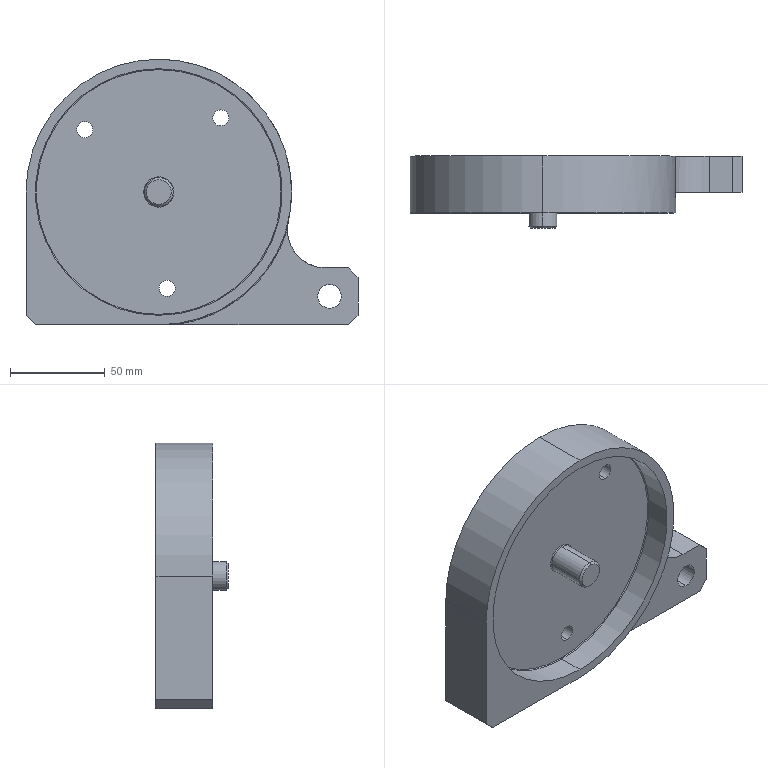Part | SolidWorks | features ICE 5, HoleWzd 2, Chamfer 1, Fillet 1, FlatPattern 1, SMBaseFlange 1, SheetMetal 1 | 1 solid | 49 faces | box 175 x 38 x 140 mm | volume 313299 mm3 | cylinder 21 | plane 13 | cone 8 | torus 7 | commonest cylinder face diameters 8.5 x10 12.5 x2 15 x2 83 x2 130 x2 140 x2
STEP:
#1=CARTESIAN_POINT('',(70.,-5.5,29.));
#2=VERTEX_POINT('',#1);
#3=CARTESIAN_POINT('',(70.,-5.5,111.));
#4=VERTEX_POINT('',#3);
#5=CARTESIAN_POINT('',(70.,-5.5,70.));
#6=DIRECTION('',(0.,1.,0.));
#7=DIRECTION('',(0.,0.,1.));
#8=AXIS2_PLACEMENT_3D('',#5,#6,#7);
#9=CIRCLE('',#8,41.);
#10=EDGE_CURVE('',#2,#4,#9,.T.);
#11=ORIENTED_EDGE('',*,*,#10,.F.);
#12=CARTESIAN_POINT('',(70.,-5.,28.5));
#13=VERTEX_POINT('',#12);
#14=CARTESIAN_POINT('',(70.,-5.,29.));
#15=DIRECTION('',(1.,0.,0.));
#16=DIRECTION('',(0.,0.,-1.));
#17=AXIS2_PLACEMENT_3D('',#14,#15,#16);
#18=CIRCLE('',#17,0.5);
#19=EDGE_CURVE('',#2,#13,#18,.T.);
#20=ORIENTED_EDGE('',*,*,#19,.T.);
#21=CARTESIAN_POINT('',(70.,-5.,111.5));
#22=VERTEX_POINT('',#21);
#23=CARTESIAN_POINT('',(70.,-5.,70.));
#24=DIRECTION('',(0.,-1.,0.));
#25=DIRECTION('',(0.,0.,1.));
#26=AXIS2_PLACEMENT_3D('',#23,#24,#25);
#27=CIRCLE('',#26,41.5);
#28=EDGE_CURVE('',#22,#13,#27,.T.);
#29=ORIENTED_EDGE('',*,*,#28,.F.);
#30=CARTESIAN_POINT('',(70.,-5.,111.));
#31=DIRECTION('',(-1.,0.,0.));
#32=DIRECTION('',(0.,0.,1.));
#33=AXIS2_PLACEMENT_3D('',#30,#31,#32);
#34=CIRCLE('',#33,0.5);
#35=EDGE_CURVE('',#4,#22,#34,.T.);
#36=ORIENTED_EDGE('',*,*,#35,.F.);
#37=EDGE_LOOP('',(#11,#20,#29,#36));
#38=FACE_OUTER_BOUND('',#37,.T.);
#39=CARTESIAN_POINT('',(70.,-5.,70.));
#40=DIRECTION('',(0.,1.,0.));
#41=DIRECTION('',(0.,0.,1.));
#42=AXIS2_PLACEMENT_3D('',#39,#40,#41);
#43=TOROIDAL_SURFACE('',#42,41.,0.5);
#44=ADVANCED_FACE('',(#38),#43,.F.);
#45=CARTESIAN_POINT('',(70.,-16.,134.5));
#46=VERTEX_POINT('',#45);
#47=CARTESIAN_POINT('',(70.,-16.,5.5));
#48=VERTEX_POINT('',#47);
#49=CARTESIAN_POINT('',(70.,-16.,70.));
#50=DIRECTION('',(0.,-1.,0.));
#51=DIRECTION('',(0.,0.,-1.));
#52=AXIS2_PLACEMENT_3D('',#49,#50,#51);
#53=CIRCLE('',#52,64.5);
#54=EDGE_CURVE('',#46,#48,#53,.T.);
#55=ORIENTED_EDGE('',*,*,#54,.F.);
#56=CARTESIAN_POINT('',(70.,-16.5,135.));
#57=VERTEX_POINT('',#56);
#58=CARTESIAN_POINT('',(70.,-16.5,134.5));
#59=DIRECTION('',(1.,0.,0.));
#60=DIRECTION('',(0.,0.,-1.));
#61=AXIS2_PLACEMENT_3D('',#58,#59,#60);
#62=CIRCLE('',#61,0.5);
#63=EDGE_CURVE('',#46,#57,#62,.T.);
#64=ORIENTED_EDGE('',*,*,#63,.T.);
#65=CARTESIAN_POINT('',(70.,-16.5,5.));
#66=VERTEX_POINT('',#65);
#67=CARTESIAN_POINT('',(70.,-16.5,70.));
#68=DIRECTION('',(0.,1.,0.));
#69=DIRECTION('',(0.,0.,-1.));
#70=AXIS2_PLACEMENT_3D('',#67,#68,#69);
#71=CIRCLE('',#70,65.);
#72=EDGE_CURVE('',#66,#57,#71,.T.);
#73=ORIENTED_EDGE('',*,*,#72,.F.);
#74=CARTESIAN_POINT('',(70.,-16.5,5.5));
#75=DIRECTION('',(-1.,0.,0.));
#76=DIRECTION('',(0.,0.,1.));
#77=AXIS2_PLACEMENT_3D('',#74,#75,#76);
#78=CIRCLE('',#77,0.5);
#79=EDGE_CURVE('',#48,#66,#78,.T.);
#80=ORIENTED_EDGE('',*,*,#79,.F.);
#81=EDGE_LOOP('',(#55,#64,#73,#80));
#82=FACE_OUTER_BOUND('',#81,.T.);
#83=CARTESIAN_POINT('',(70.,-16.5,70.));
#84=DIRECTION('',(0.,-1.,0.));
#85=DIRECTION('',(0.,0.,-1.));
#86=AXIS2_PLACEMENT_3D('',#83,#84,#85);
#87=TOROIDAL_SURFACE('',#86,64.5,0.5);
#88=ADVANCED_FACE('',(#82),#87,.F.);
#89=CARTESIAN_POINT('',(70.,-16.5,77.5));
#90=VERTEX_POINT('',#89);
#91=CARTESIAN_POINT('',(70.,-16.5,62.5));
#92=VERTEX_POINT('',#91);
#93=CARTESIAN_POINT('',(70.,-16.5,70.));
#94=DIRECTION('',(0.,-1.,0.));
#95=DIRECTION('',(0.,0.,-1.));
#96=AXIS2_PLACEMENT_3D('',#93,#94,#95);
#97=CIRCLE('',#96,7.5);
#98=EDGE_CURVE('',#90,#92,#97,.T.);
#99=ORIENTED_EDGE('',*,*,#98,.F.);
#100=CARTESIAN_POINT('',(70.,-16.,78.));
#101=VERTEX_POINT('',#100);
#102=CARTESIAN_POINT('',(70.,-16.5,78.));
#103=DIRECTION('',(1.,0.,0.));
#104=DIRECTION('',(0.,0.,-1.));
#105=AXIS2_PLACEMENT_3D('',#102,#103,#104);
#106=CIRCLE('',#105,0.5);
#107=EDGE_CURVE('',#90,#101,#106,.T.);
#108=ORIENTED_EDGE('',*,*,#107,.T.);
#109=CARTESIAN_POINT('',(70.,-16.,62.));
#110=VERTEX_POINT('',#109);
#111=CARTESIAN_POINT('',(70.,-16.,70.));
#112=DIRECTION('',(0.,1.,0.));
#113=DIRECTION('',(0.,0.,-1.));
#114=AXIS2_PLACEMENT_3D('',#111,#112,#113);
#115=CIRCLE('',#114,8.);
#116=EDGE_CURVE('',#110,#101,#115,.T.);
#117=ORIENTED_EDGE('',*,*,#116,.F.);
#118=CARTESIAN_POINT('',(70.,-16.5,62.));
#119=DIRECTION('',(-1.,0.,0.));
#120=DIRECTION('',(0.,0.,1.));
#121=AXIS2_PLACEMENT_3D('',#118,#119,#120);
#122=CIRCLE('',#121,0.5);
#123=EDGE_CURVE('',#92,#110,#122,.T.);
#124=ORIENTED_EDGE('',*,*,#123,.F.);
#125=EDGE_LOOP('',(#99,#108,#117,#124));
#126=FACE_OUTER_BOUND('',#125,.T.);
#127=CARTESIAN_POINT('',(70.,-16.5,70.));
#128=DIRECTION('',(0.,-1.,0.));
#129=DIRECTION('',(0.,0.,-1.));
#130=AXIS2_PLACEMENT_3D('',#127,#128,#129);
#131=TOROIDAL_SURFACE('',#130,8.,0.5);
#132=ADVANCED_FACE('',(#126),#131,.F.);
#133=CARTESIAN_POINT('',(70.,-1.,28.5));
#134=VERTEX_POINT('',#133);
#135=CARTESIAN_POINT('',(70.,-1.,111.5));
#136=VERTEX_POINT('',#135);
#137=CARTESIAN_POINT('',(70.,-1.,70.));
#138=DIRECTION('',(0.,1.,0.));
#139=DIRECTION('',(0.,0.,-1.));
#140=AXIS2_PLACEMENT_3D('',#137,#138,#139);
#141=CIRCLE('',#140,41.5);
#142=EDGE_CURVE('',#134,#136,#141,.T.);
#143=ORIENTED_EDGE('',*,*,#142,.F.);
#144=CARTESIAN_POINT('',(70.,0.,27.5));
#145=VERTEX_POINT('',#144);
#146=CARTESIAN_POINT('',(70.,-1.,28.5));
#147=DIRECTION('',(0.,0.7071,-0.7071));
#148=VECTOR('',#147,1000.);
#149=LINE('',#146,#148);
#150=EDGE_CURVE('',#134,#145,#149,.T.);
#151=ORIENTED_EDGE('',*,*,#150,.T.);
#152=CARTESIAN_POINT('',(70.,0.,112.5));
#153=VERTEX_POINT('',#152);
#154=CARTESIAN_POINT('',(70.,0.,70.));
#155=DIRECTION('',(0.,-1.,0.));
#156=DIRECTION('',(0.,0.,-1.));
#157=AXIS2_PLACEMENT_3D('',#154,#155,#156);
#158=CIRCLE('',#157,42.5);
#159=EDGE_CURVE('',#153,#145,#158,.T.);
#160=ORIENTED_EDGE('',*,*,#159,.F.);
#161=CARTESIAN_POINT('',(70.,-1.,111.5));
#162=DIRECTION('',(0.,0.7071,0.7071));
#163=VECTOR('',#162,1000.);
#164=LINE('',#161,#163);
#165=EDGE_CURVE('',#136,#153,#164,.T.);
#166=ORIENTED_EDGE('',*,*,#165,.F.);
#167=EDGE_LOOP('',(#143,#151,#160,#166));
#168=FACE_OUTER_BOUND('',#167,.T.);
#169=CARTESIAN_POINT('',(70.,-1.,70.));
#170=DIRECTION('',(0.,1.,0.));
#171=DIRECTION('',(0.,0.,1.));
#172=AXIS2_PLACEMENT_3D('',#169,#170,#171);
#173=CONICAL_SURFACE('',#172,41.5,0.7854);
#174=ADVANCED_FACE('',(#168),#173,.F.);
#175=CARTESIAN_POINT('',(70.,-38.,63.5));
#176=VERTEX_POINT('',#175);
#177=CARTESIAN_POINT('',(70.,-38.,76.5));
#178=VERTEX_POINT('',#177);
#179=CARTESIAN_POINT('',(70.,-38.,70.));
#180=DIRECTION('',(0.,-1.,0.));
#181=DIRECTION('',(0.,0.,-1.));
#182=AXIS2_PLACEMENT_3D('',#179,#180,#181);
#183=CIRCLE('',#182,6.5);
#184=EDGE_CURVE('',#176,#178,#183,.T.);
#185=ORIENTED_EDGE('',*,*,#184,.F.);
#186=CARTESIAN_POINT('',(70.,-37.,62.5));
#187=VERTEX_POINT('',#186);
#188=CARTESIAN_POINT('',(70.,-38.,63.5));
#189=DIRECTION('',(0.,0.7071,-0.7071));
#190=VECTOR('',#189,1000.);
#191=LINE('',#188,#190);
#192=EDGE_CURVE('',#176,#187,#191,.T.);
#193=ORIENTED_EDGE('',*,*,#192,.T.);
#194=CARTESIAN_POINT('',(70.,-37.,77.5));
#195=VERTEX_POINT('',#194);
#196=CARTESIAN_POINT('',(70.,-37.,70.));
#197=DIRECTION('',(0.,1.,0.));
#198=DIRECTION('',(0.,0.,-1.));
#199=AXIS2_PLACEMENT_3D('',#196,#197,#198);
#200=CIRCLE('',#199,7.5);
#201=EDGE_CURVE('',#195,#187,#200,.T.);
#202=ORIENTED_EDGE('',*,*,#201,.F.);
#203=CARTESIAN_POINT('',(70.,-38.,76.5));
#204=DIRECTION('',(0.,0.7071,0.7071));
#205=VECTOR('',#204,1000.);
#206=LINE('',#203,#205);
#207=EDGE_CURVE('',#178,#195,#206,.T.);
#208=ORIENTED_EDGE('',*,*,#207,.F.);
#209=EDGE_LOOP('',(#185,#193,#202,#208));
#210=FACE_OUTER_BOUND('',#209,.T.);
#211=CARTESIAN_POINT('',(70.,-38.,70.));
#212=DIRECTION('',(0.,1.,0.));
#213=DIRECTION('',(0.,0.,1.));
#214=AXIS2_PLACEMENT_3D('',#211,#212,#213);
#215=CONICAL_SURFACE('',#214,6.5,0.7854);
#216=ADVANCED_FACE('',(#210),#215,.T.);
#217=CARTESIAN_POINT('',(19.25,-9.5,23.));
#218=VERTEX_POINT('',#217);
#219=CARTESIAN_POINT('',(10.75,-9.5,23.));
#220=VERTEX_POINT('',#219);
#221=CARTESIAN_POINT('',(15.,-9.5,23.));
#222=DIRECTION('',(0.,0.,-1.));
#223=DIRECTION('',(-1.,0.,0.));
#224=AXIS2_PLACEMENT_3D('',#221,#222,#223);
#225=CIRCLE('',#224,4.25);
#226=EDGE_CURVE('',#218,#220,#225,.T.);
#227=ORIENTED_EDGE('',*,*,#226,.F.);
#228=CARTESIAN_POINT('',(19.25,-9.5,0.));
#229=VERTEX_POINT('',#228);
#230=CARTESIAN_POINT('',(19.25,-9.5,0.));
#231=DIRECTION('',(0.,0.,-1.));
#232=VECTOR('',#231,1000.);
#233=LINE('',#230,#232);
#234=EDGE_CURVE('',#218,#229,#233,.T.);
#235=ORIENTED_EDGE('',*,*,#234,.T.);
#236=CARTESIAN_POINT('',(10.75,-9.5,0.));
#237=VERTEX_POINT('',#236);
#238=CARTESIAN_POINT('',(15.,-9.5,0.));
#239=DIRECTION('',(0.,0.,-1.));
#240=DIRECTION('',(-1.,0.,0.));
#241=AXIS2_PLACEMENT_3D('',#238,#239,#240);
#242=CIRCLE('',#241,4.25);
#243=EDGE_CURVE('',#229,#237,#242,.T.);
#244=ORIENTED_EDGE('',*,*,#243,.T.);
#245=CARTESIAN_POINT('',(10.75,-9.5,0.));
#246=DIRECTION('',(0.,0.,-1.));
#247=VECTOR('',#246,1000.);
#248=LINE('',#245,#247);
#249=EDGE_CURVE('',#220,#237,#248,.T.);
#250=ORIENTED_EDGE('',*,*,#249,.F.);
#251=EDGE_LOOP('',(#227,#235,#244,#250));
#252=FACE_OUTER_BOUND('',#251,.T.);
#253=CARTESIAN_POINT('',(15.,-9.5,0.));
#254=DIRECTION('',(0.,0.,-1.));
#255=DIRECTION('',(-1.,0.,0.));
#256=AXIS2_PLACEMENT_3D('',#253,#254,#255);
#257=CYLINDRICAL_SURFACE('',#256,4.25);
#258=ADVANCED_FACE('',(#252),#257,.F.);
#259=CARTESIAN_POINT('',(15.,-9.5,25.554));
#260=VERTEX_POINT('',#259);
#261=CARTESIAN_POINT('',(10.75,-9.5,23.));
#262=DIRECTION('',(-0.8572,0.,-0.515));
#263=VECTOR('',#262,1000.);
#264=LINE('',#261,#263);
#265=EDGE_CURVE('',#260,#220,#264,.T.);
#266=ORIENTED_EDGE('',*,*,#265,.F.);
#267=CARTESIAN_POINT('',(19.25,-9.5,23.));
#268=DIRECTION('',(0.8572,0.,-0.515));
#269=VECTOR('',#268,1000.);
#270=LINE('',#267,#269);
#271=EDGE_CURVE('',#260,#218,#270,.T.);
#272=ORIENTED_EDGE('',*,*,#271,.T.);
#273=ORIENTED_EDGE('',*,*,#226,.T.);
#274=EDGE_LOOP('',(#266,#272,#273));
#275=FACE_OUTER_BOUND('',#274,.T.);
#276=CARTESIAN_POINT('',(15.,-9.5,23.));
#277=DIRECTION('',(0.,0.,-1.));
#278=DIRECTION('',(-1.,0.,0.));
#279=AXIS2_PLACEMENT_3D('',#276,#277,#278);
#280=CONICAL_SURFACE('',#279,4.25,1.03);
#281=ADVANCED_FACE('',(#275),#280,.F.);
#282=CARTESIAN_POINT('',(134.25,-9.5,23.));
#283=VERTEX_POINT('',#282);
#284=CARTESIAN_POINT('',(125.75,-9.5,23.));
#285=VERTEX_POINT('',#284);
#286=CARTESIAN_POINT('',(130.,-9.5,23.));
#287=DIRECTION('',(0.,0.,-1.));
#288=DIRECTION('',(-1.,0.,0.));
#289=AXIS2_PLACEMENT_3D('',#286,#287,#288);
#290=CIRCLE('',#289,4.25);
#291=EDGE_CURVE('',#283,#285,#290,.T.);
#292=ORIENTED_EDGE('',*,*,#291,.F.);
#293=CARTESIAN_POINT('',(134.25,-9.5,0.));
#294=VERTEX_POINT('',#293);
#295=CARTESIAN_POINT('',(134.25,-9.5,0.));
#296=DIRECTION('',(0.,0.,-1.));
#297=VECTOR('',#296,1000.);
#298=LINE('',#295,#297);
#299=EDGE_CURVE('',#283,#294,#298,.T.);
#300=ORIENTED_EDGE('',*,*,#299,.T.);
#301=CARTESIAN_POINT('',(125.75,-9.5,0.));
#302=VERTEX_POINT('',#301);
#303=CARTESIAN_POINT('',(130.,-9.5,0.));
#304=DIRECTION('',(0.,0.,-1.));
#305=DIRECTION('',(-1.,0.,0.));
#306=AXIS2_PLACEMENT_3D('',#303,#304,#305);
#307=CIRCLE('',#306,4.25);
#308=EDGE_CURVE('',#294,#302,#307,.T.);
#309=ORIENTED_EDGE('',*,*,#308,.T.);
#310=CARTESIAN_POINT('',(125.75,-9.5,0.));
#311=DIRECTION('',(0.,0.,-1.));
#312=VECTOR('',#311,1000.);
#313=LINE('',#310,#312);
#314=EDGE_CURVE('',#285,#302,#313,.T.);
#315=ORIENTED_EDGE('',*,*,#314,.F.);
#316=EDGE_LOOP('',(#292,#300,#309,#315));
#317=FACE_OUTER_BOUND('',#316,.T.);
#318=CARTESIAN_POINT('',(130.,-9.5,0.));
#319=DIRECTION('',(0.,0.,-1.));
#320=DIRECTION('',(-1.,0.,0.));
#321=AXIS2_PLACEMENT_3D('',#318,#319,#320);
#322=CYLINDRICAL_SURFACE('',#321,4.25);
#323=ADVANCED_FACE('',(#317),#322,.F.);
#324=CARTESIAN_POINT('',(130.,-9.5,25.554));
#325=VERTEX_POINT('',#324);
#326=CARTESIAN_POINT('',(125.75,-9.5,23.));
#327=DIRECTION('',(-0.8572,0.,-0.515));
#328=VECTOR('',#327,1000.);
#329=LINE('',#326,#328);
#330=EDGE_CURVE('',#325,#285,#329,.T.);
#331=ORIENTED_EDGE('',*,*,#330,.F.);
#332=CARTESIAN_POINT('',(134.25,-9.5,23.));
#333=DIRECTION('',(0.8572,0.,-0.515));
#334=VECTOR('',#333,1000.);
#335=LINE('',#332,#334);
#336=EDGE_CURVE('',#325,#283,#335,.T.);
#337=ORIENTED_EDGE('',*,*,#336,.T.);
#338=ORIENTED_EDGE('',*,*,#291,.T.);
#339=EDGE_LOOP('',(#331,#337,#338));
#340=FACE_OUTER_BOUND('',#339,.T.);
#341=CARTESIAN_POINT('',(130.,-9.5,23.));
#342=DIRECTION('',(0.,0.,-1.));
#343=DIRECTION('',(-1.,0.,0.));
#344=AXIS2_PLACEMENT_3D('',#341,#342,#343);
#345=CONICAL_SURFACE('',#344,4.25,1.03);
#346=ADVANCED_FACE('',(#340),#345,.F.);
#347=CARTESIAN_POINT('',(102.782,-16.,113.318));
#348=VERTEX_POINT('',#347);
#349=CARTESIAN_POINT('',(102.782,-16.,104.818));
#350=VERTEX_POINT('',#349);
#351=CARTESIAN_POINT('',(102.782,-16.,109.068));
#352=DIRECTION('',(0.,-1.,0.));
#353=DIRECTION('',(0.,0.,-1.));
#354=AXIS2_PLACEMENT_3D('',#351,#352,#353);
#355=CIRCLE('',#354,4.25);
#356=EDGE_CURVE('',#348,#350,#355,.T.);
#357=ORIENTED_EDGE('',*,*,#356,.T.);
#358=CARTESIAN_POINT('',(102.782,0.,104.818));
#359=VERTEX_POINT('',#358);
#360=CARTESIAN_POINT('',(102.782,0.,104.818));
#361=DIRECTION('',(0.,1.,0.));
#362=VECTOR('',#361,1000.);
#363=LINE('',#360,#362);
#364=EDGE_CURVE('',#350,#359,#363,.T.);
#365=ORIENTED_EDGE('',*,*,#364,.T.);
#366=CARTESIAN_POINT('',(102.782,0.,113.318));
#367=VERTEX_POINT('',#366);
#368=CARTESIAN_POINT('',(102.782,0.,109.068));
#369=DIRECTION('',(0.,1.,0.));
#370=DIRECTION('',(0.,0.,1.));
#371=AXIS2_PLACEMENT_3D('',#368,#369,#370);
#372=CIRCLE('',#371,4.25);
#373=EDGE_CURVE('',#359,#367,#372,.T.);
#374=ORIENTED_EDGE('',*,*,#373,.T.);
#375=CARTESIAN_POINT('',(102.782,0.,113.318));
#376=DIRECTION('',(0.,1.,0.));
#377=VECTOR('',#376,1000.);
#378=LINE('',#375,#377);
#379=EDGE_CURVE('',#348,#367,#378,.T.);
#380=ORIENTED_EDGE('',*,*,#379,.F.);
#381=EDGE_LOOP('',(#357,#365,#374,#380));
#382=FACE_OUTER_BOUND('',#381,.T.);
#383=CARTESIAN_POINT('',(102.782,0.,109.068));
#384=DIRECTION('',(0.,1.,0.));
#385=DIRECTION('',(0.,0.,1.));
#386=AXIS2_PLACEMENT_3D('',#383,#384,#385);
#387=CYLINDRICAL_SURFACE('',#386,4.25);
#388=ADVANCED_FACE('',(#382),#387,.F.);
#389=CARTESIAN_POINT('',(74.445,-16.,23.444));
#390=VERTEX_POINT('',#389);
#391=CARTESIAN_POINT('',(74.445,-16.,14.944));
#392=VERTEX_POINT('',#391);
#393=CARTESIAN_POINT('',(74.445,-16.,19.194));
#394=DIRECTION('',(0.,-1.,0.));
#395=DIRECTION('',(0.,0.,-1.));
#396=AXIS2_PLACEMENT_3D('',#393,#394,#395);
#397=CIRCLE('',#396,4.25);
#398=EDGE_CURVE('',#390,#392,#397,.T.);
#399=ORIENTED_EDGE('',*,*,#398,.T.);
#400=CARTESIAN_POINT('',(74.445,0.,14.944));
#401=VERTEX_POINT('',#400);
#402=CARTESIAN_POINT('',(74.445,0.,14.944));
#403=DIRECTION('',(0.,1.,0.));
#404=VECTOR('',#403,1000.);
#405=LINE('',#402,#404);
#406=EDGE_CURVE('',#392,#401,#405,.T.);
#407=ORIENTED_EDGE('',*,*,#406,.T.);
#408=CARTESIAN_POINT('',(74.445,0.,23.444));
#409=VERTEX_POINT('',#408);
#410=CARTESIAN_POINT('',(74.445,0.,19.194));
#411=DIRECTION('',(0.,1.,0.));
#412=DIRECTION('',(0.,0.,1.));
#413=AXIS2_PLACEMENT_3D('',#410,#411,#412);
#414=CIRCLE('',#413,4.25);
#415=EDGE_CURVE('',#401,#409,#414,.T.);
#416=ORIENTED_EDGE('',*,*,#415,.T.);
#417=CARTESIAN_POINT('',(74.445,0.,23.444));
#418=DIRECTION('',(0.,1.,0.));
#419=VECTOR('',#418,1000.);
#420=LINE('',#417,#419);
#421=EDGE_CURVE('',#390,#409,#420,.T.);
#422=ORIENTED_EDGE('',*,*,#421,.F.);
#423=EDGE_LOOP('',(#399,#407,#416,#422));
#424=FACE_OUTER_BOUND('',#423,.T.);
#425=CARTESIAN_POINT('',(74.445,0.,19.194));
#426=DIRECTION('',(0.,1.,0.));
#427=DIRECTION('',(0.,0.,1.));
#428=AXIS2_PLACEMENT_3D('',#425,#426,#427);
#429=CYLINDRICAL_SURFACE('',#428,4.25);
#430=ADVANCED_FACE('',(#424),#429,.F.);
#431=CARTESIAN_POINT('',(30.932,-16.,107.032));
#432=VERTEX_POINT('',#431);
#433=CARTESIAN_POINT('',(30.932,-16.,98.532));
#434=VERTEX_POINT('',#433);
#435=CARTESIAN_POINT('',(30.932,-16.,102.782));
#436=DIRECTION('',(0.,-1.,0.));
#437=DIRECTION('',(0.,0.,-1.));
#438=AXIS2_PLACEMENT_3D('',#435,#436,#437);
#439=CIRCLE('',#438,4.25);
#440=EDGE_CURVE('',#432,#434,#439,.T.);
#441=ORIENTED_EDGE('',*,*,#440,.T.);
#442=CARTESIAN_POINT('',(30.932,0.,98.532));
#443=VERTEX_POINT('',#442);
#444=CARTESIAN_POINT('',(30.932,0.,98.532));
#445=DIRECTION('',(0.,1.,0.));
#446=VECTOR('',#445,1000.);
#447=LINE('',#444,#446);
#448=EDGE_CURVE('',#434,#443,#447,.T.);
#449=ORIENTED_EDGE('',*,*,#448,.T.);
#450=CARTESIAN_POINT('',(30.932,0.,107.032));
#451=VERTEX_POINT('',#450);
#452=CARTESIAN_POINT('',(30.932,0.,102.782));
#453=DIRECTION('',(0.,1.,0.));
#454=DIRECTION('',(0.,0.,1.));
#455=AXIS2_PLACEMENT_3D('',#452,#453,#454);
#456=CIRCLE('',#455,4.25);
#457=EDGE_CURVE('',#443,#451,#456,.T.);
#458=ORIENTED_EDGE('',*,*,#457,.T.);
#459=CARTESIAN_POINT('',(30.932,0.,107.032));
#460=DIRECTION('',(0.,1.,0.));
#461=VECTOR('',#460,1000.);
#462=LINE('',#459,#461);
#463=EDGE_CURVE('',#432,#451,#462,.T.);
#464=ORIENTED_EDGE('',*,*,#463,.F.);
#465=EDGE_LOOP('',(#441,#449,#458,#464));
#466=FACE_OUTER_BOUND('',#465,.T.);
#467=CARTESIAN_POINT('',(30.932,0.,102.782));
#468=DIRECTION('',(0.,1.,0.));
#469=DIRECTION('',(0.,0.,1.));
#470=AXIS2_PLACEMENT_3D('',#467,#468,#469);
#471=CYLINDRICAL_SURFACE('',#470,4.25);
#472=ADVANCED_FACE('',(#466),#471,.F.);
#473=ORIENTED_EDGE('',*,*,#28,.T.);
#474=CARTESIAN_POINT('',(70.,-5.5,28.5));
#475=DIRECTION('',(0.,1.,0.));
#476=VECTOR('',#475,1000.);
#477=LINE('',#474,#476);
#478=EDGE_CURVE('',#13,#134,#477,.T.);
#479=ORIENTED_EDGE('',*,*,#478,.T.);
#480=ORIENTED_EDGE('',*,*,#142,.T.);
#481=CARTESIAN_POINT('',(70.,-5.5,111.5));
#482=DIRECTION('',(0.,1.,0.));
#483=VECTOR('',#482,1000.);
#484=LINE('',#481,#483);
#485=EDGE_CURVE('',#22,#136,#484,.T.);
#486=ORIENTED_EDGE('',*,*,#485,.F.);
#487=EDGE_LOOP('',(#473,#479,#480,#486));
#488=FACE_OUTER_BOUND('',#487,.T.);
#489=CARTESIAN_POINT('',(70.,-5.5,70.));
#490=DIRECTION('',(0.,1.,0.));
#491=DIRECTION('',(0.,0.,1.));
#492=AXIS2_PLACEMENT_3D('',#489,#490,#491);
#493=CYLINDRICAL_SURFACE('',#492,41.5);
#494=ADVANCED_FACE('',(#488),#493,.F.);
#495=CARTESIAN_POINT('',(70.,-16.5,70.));
#496=DIRECTION('',(0.,-1.,0.));
#497=DIRECTION('',(0.,0.,-1.));
#498=AXIS2_PLACEMENT_3D('',#495,#496,#497);
#499=CIRCLE('',#498,7.5);
#500=EDGE_CURVE('',#92,#90,#499,.T.);
#501=ORIENTED_EDGE('',*,*,#500,.T.);
#502=CARTESIAN_POINT('',(70.,-16.,77.5));
#503=DIRECTION('',(0.,-1.,0.));
#504=VECTOR('',#503,1000.);
#505=LINE('',#502,#504);
#506=EDGE_CURVE('',#90,#195,#505,.T.);
#507=ORIENTED_EDGE('',*,*,#506,.T.);
#508=ORIENTED_EDGE('',*,*,#201,.T.);
#509=CARTESIAN_POINT('',(70.,-16.,62.5));
#510=DIRECTION('',(0.,-1.,0.));
#511=VECTOR('',#510,1000.);
#512=LINE('',#509,#511);
#513=EDGE_CURVE('',#92,#187,#512,.T.);
#514=ORIENTED_EDGE('',*,*,#513,.F.);
#515=EDGE_LOOP('',(#501,#507,#508,#514));
#516=FACE_OUTER_BOUND('',#515,.T.);
#517=CARTESIAN_POINT('',(70.,-16.,70.));
#518=DIRECTION('',(0.,-1.,0.));
#519=DIRECTION('',(0.,0.,-1.));
#520=AXIS2_PLACEMENT_3D('',#517,#518,#519);
#521=CYLINDRICAL_SURFACE('',#520,7.5);
#522=ADVANCED_FACE('',(#516),#521,.T.);
#523=ORIENTED_EDGE('',*,*,#72,.T.);
#524=CARTESIAN_POINT('',(70.,-30.,135.));
#525=VERTEX_POINT('',#524);
#526=CARTESIAN_POINT('',(70.,-16.,135.));
#527=DIRECTION('',(0.,-1.,0.));
#528=VECTOR('',#527,1000.);
#529=LINE('',#526,#528);
#530=EDGE_CURVE('',#57,#525,#529,.T.);
#531=ORIENTED_EDGE('',*,*,#530,.T.);
#532=CARTESIAN_POINT('',(70.,-30.,5.));
#533=VERTEX_POINT('',#532);
#534=CARTESIAN_POINT('',(70.,-30.,70.));
#535=DIRECTION('',(0.,-1.,0.));
#536=DIRECTION('',(0.,0.,-1.));
#537=AXIS2_PLACEMENT_3D('',#534,#535,#536);
#538=CIRCLE('',#537,65.);
#539=EDGE_CURVE('',#525,#533,#538,.T.);
#540=ORIENTED_EDGE('',*,*,#539,.T.);
#541=CARTESIAN_POINT('',(70.,-16.,5.));
#542=DIRECTION('',(0.,-1.,0.));
#543=VECTOR('',#542,1000.);
#544=LINE('',#541,#543);
#545=EDGE_CURVE('',#66,#533,#544,.T.);
#546=ORIENTED_EDGE('',*,*,#545,.F.);
#547=EDGE_LOOP('',(#523,#531,#540,#546));
#548=FACE_OUTER_BOUND('',#547,.T.);
#549=CARTESIAN_POINT('',(70.,-16.,70.));
#550=DIRECTION('',(0.,-1.,0.));
#551=DIRECTION('',(0.,0.,-1.));
#552=AXIS2_PLACEMENT_3D('',#549,#550,#551);
#553=CYLINDRICAL_SURFACE('',#552,65.);
#554=ADVANCED_FACE('',(#548),#553,.F.);
#555=CARTESIAN_POINT('',(0.,-30.,70.));
#556=VERTEX_POINT('',#555);
#557=CARTESIAN_POINT('',(70.,-30.,140.));
#558=VERTEX_POINT('',#557);
#559=CARTESIAN_POINT('',(70.,-30.,70.));
#560=DIRECTION('',(0.,1.,0.));
#561=DIRECTION('',(0.,0.,1.));
#562=AXIS2_PLACEMENT_3D('',#559,#560,#561);
#563=CIRCLE('',#562,70.);
#564=EDGE_CURVE('',#556,#558,#563,.T.);
#565=ORIENTED_EDGE('',*,*,#564,.T.);
#566=CARTESIAN_POINT('',(70.,0.,140.));
#567=VERTEX_POINT('',#566);
#568=CARTESIAN_POINT('',(70.,-30.,140.));
#569=DIRECTION('',(0.,1.,0.));
#570=VECTOR('',#569,1000.);
#571=LINE('',#568,#570);
#572=EDGE_CURVE('',#558,#567,#571,.T.);
#573=ORIENTED_EDGE('',*,*,#572,.T.);
#574=CARTESIAN_POINT('',(0.,0.,70.));
#575=VERTEX_POINT('',#574);
#576=CARTESIAN_POINT('',(70.,0.,70.));
#577=DIRECTION('',(0.,1.,0.));
#578=DIRECTION('',(0.,0.,1.));
#579=AXIS2_PLACEMENT_3D('',#576,#577,#578);
#580=CIRCLE('',#579,70.);
#581=EDGE_CURVE('',#575,#567,#580,.T.);
#582=ORIENTED_EDGE('',*,*,#581,.F.);
#583=CARTESIAN_POINT('',(0.,-30.,70.));
#584=DIRECTION('',(0.,1.,0.));
#585=VECTOR('',#584,1000.);
#586=LINE('',#583,#585);
#587=EDGE_CURVE('',#556,#575,#586,.T.);
#588=ORIENTED_EDGE('',*,*,#587,.F.);
#589=EDGE_LOOP('',(#565,#573,#582,#588));
#590=FACE_OUTER_BOUND('',#589,.T.);
#591=CARTESIAN_POINT('',(70.,-30.,70.));
#592=DIRECTION('',(0.,1.,0.));
#593=DIRECTION('',(0.,0.,1.));
#594=AXIS2_PLACEMENT_3D('',#591,#592,#593);
#595=CYLINDRICAL_SURFACE('',#594,70.);
#596=ADVANCED_FACE('',(#590),#595,.T.);
#597=CARTESIAN_POINT('',(160.,-19.,8.75));
#598=VERTEX_POINT('',#597);
#599=CARTESIAN_POINT('',(160.,-19.,21.25));
#600=VERTEX_POINT('',#599);
#601=CARTESIAN_POINT('',(160.,-19.,15.));
#602=DIRECTION('',(0.,1.,0.));
#603=DIRECTION('',(0.,0.,-1.));
#604=AXIS2_PLACEMENT_3D('',#601,#602,#603);
#605=CIRCLE('',#604,6.25);
#606=EDGE_CURVE('',#598,#600,#605,.T.);
#607=ORIENTED_EDGE('',*,*,#606,.F.);
#608=CARTESIAN_POINT('',(160.,0.,8.75));
#609=VERTEX_POINT('',#608);
#610=CARTESIAN_POINT('',(160.,-30.,8.75));
#611=DIRECTION('',(0.,1.,0.));
#612=VECTOR('',#611,1000.);
#613=LINE('',#610,#612);
#614=EDGE_CURVE('',#598,#609,#613,.T.);
#615=ORIENTED_EDGE('',*,*,#614,.T.);
#616=CARTESIAN_POINT('',(160.,0.,21.25));
#617=VERTEX_POINT('',#616);
#618=CARTESIAN_POINT('',(160.,0.,15.));
#619=DIRECTION('',(0.,1.,0.));
#620=DIRECTION('',(0.,0.,1.));
#621=AXIS2_PLACEMENT_3D('',#618,#619,#620);
#622=CIRCLE('',#621,6.25);
#623=EDGE_CURVE('',#609,#617,#622,.T.);
#624=ORIENTED_EDGE('',*,*,#623,.T.);
#625=CARTESIAN_POINT('',(160.,-30.,21.25));
#626=DIRECTION('',(0.,1.,0.));
#627=VECTOR('',#626,1000.);
#628=LINE('',#625,#627);
#629=EDGE_CURVE('',#600,#617,#628,.T.);
#630=ORIENTED_EDGE('',*,*,#629,.F.);
#631=EDGE_LOOP('',(#607,#615,#624,#630));
#632=FACE_OUTER_BOUND('',#631,.T.);
#633=CARTESIAN_POINT('',(160.,-30.,15.));
#634=DIRECTION('',(0.,1.,0.));
#635=DIRECTION('',(0.,0.,1.));
#636=AXIS2_PLACEMENT_3D('',#633,#634,#635);
#637=CYLINDRICAL_SURFACE('',#636,6.25);
#638=ADVANCED_FACE('',(#632),#637,.F.);
#639=CARTESIAN_POINT('',(138.25,-19.5,54.444));
#640=VERTEX_POINT('',#639);
#641=CARTESIAN_POINT('',(138.25,0.,54.444));
#642=VERTEX_POINT('',#641);
#643=CARTESIAN_POINT('',(138.25,-30.,54.444));
#644=DIRECTION('',(0.,1.,0.));
#645=VECTOR('',#644,1000.);
#646=LINE('',#643,#645);
#647=EDGE_CURVE('',#640,#642,#646,.T.);
#648=ORIENTED_EDGE('',*,*,#647,.F.);
#649=CARTESIAN_POINT('',(137.757,-19.,50.524));
#650=VERTEX_POINT('',#649);
#651=CARTESIAN_POINT('',(138.25,-19.5,54.444));
#652=CARTESIAN_POINT('',(138.104,-19.383,53.807));
#653=CARTESIAN_POINT('',(137.99,-19.265,53.16));
#654=CARTESIAN_POINT('',(137.866,-19.123,52.181));
#655=CARTESIAN_POINT('',(137.833,-19.082,51.853));
#656=CARTESIAN_POINT('',(137.782,-19.02,51.19));
#657=CARTESIAN_POINT('',(137.765,-19.,50.858));
#658=CARTESIAN_POINT('',(137.757,-19.,50.524));
#659=B_SPLINE_CURVE_WITH_KNOTS('',3,(#651,#652,#653,#654,#655,#656,#657,#658),.UNSPECIFIED.,.F.,.F.,(4,2,2,4),(-0.00002494,0.001968,0.002965,0.003962),.UNSPECIFIED.);
#660=EDGE_CURVE('',#640,#650,#659,.T.);
#661=ORIENTED_EDGE('',*,*,#660,.T.);
#662=CARTESIAN_POINT('',(157.75,-19.,30.));
#663=VERTEX_POINT('',#662);
#664=CARTESIAN_POINT('',(157.75,-19.,50.));
#665=DIRECTION('',(0.,1.,0.));
#666=DIRECTION('',(0.,0.,-1.));
#667=AXIS2_PLACEMENT_3D('',#664,#665,#666);
#668=CIRCLE('',#667,20.);
#669=EDGE_CURVE('',#663,#650,#668,.T.);
#670=ORIENTED_EDGE('',*,*,#669,.F.);
#671=CARTESIAN_POINT('',(157.75,0.,30.));
#672=VERTEX_POINT('',#671);
#673=CARTESIAN_POINT('',(157.75,-30.,30.));
#674=DIRECTION('',(0.,1.,0.));
#675=VECTOR('',#674,1000.);
#676=LINE('',#673,#675);
#677=EDGE_CURVE('',#663,#672,#676,.T.);
#678=ORIENTED_EDGE('',*,*,#677,.T.);
#679=CARTESIAN_POINT('',(157.75,0.,50.));
#680=DIRECTION('',(0.,-1.,0.));
#681=DIRECTION('',(0.,0.,-1.));
#682=AXIS2_PLACEMENT_3D('',#679,#680,#681);
#683=CIRCLE('',#682,20.);
#684=EDGE_CURVE('',#642,#672,#683,.T.);
#685=ORIENTED_EDGE('',*,*,#684,.F.);
#686=EDGE_LOOP('',(#648,#661,#670,#678,#685));
#687=FACE_OUTER_BOUND('',#686,.T.);
#688=CARTESIAN_POINT('',(157.75,-30.,50.));
#689=DIRECTION('',(0.,1.,0.));
#690=DIRECTION('',(0.,0.,1.));
#691=AXIS2_PLACEMENT_3D('',#688,#689,#690);
#692=CYLINDRICAL_SURFACE('',#691,20.);
#693=ADVANCED_FACE('',(#687),#692,.F.);
#694=CARTESIAN_POINT('',(175.,-19.,5.));
#695=VERTEX_POINT('',#694);
#696=CARTESIAN_POINT('',(175.,0.,5.));
#697=VERTEX_POINT('',#696);
#698=CARTESIAN_POINT('',(175.,-30.,5.));
#699=DIRECTION('',(0.,1.,0.));
#700=VECTOR('',#699,1000.);
#701=LINE('',#698,#700);
#702=EDGE_CURVE('',#695,#697,#701,.T.);
#703=ORIENTED_EDGE('',*,*,#702,.F.);
#704=CARTESIAN_POINT('',(170.,-19.,0.));
#705=VERTEX_POINT('',#704);
#706=CARTESIAN_POINT('',(175.,-19.,5.));
#707=DIRECTION('',(0.7071,0.,0.7071));
#708=VECTOR('',#707,1000.);
#709=LINE('',#706,#708);
#710=EDGE_CURVE('',#705,#695,#709,.T.);
#711=ORIENTED_EDGE('',*,*,#710,.F.);
#712=CARTESIAN_POINT('',(170.,0.,0.));
#713=VERTEX_POINT('',#712);
#714=CARTESIAN_POINT('',(170.,-30.,0.));
#715=DIRECTION('',(0.,1.,0.));
#716=VECTOR('',#715,1000.);
#717=LINE('',#714,#716);
#718=EDGE_CURVE('',#705,#713,#717,.T.);
#719=ORIENTED_EDGE('',*,*,#718,.T.);
#720=CARTESIAN_POINT('',(170.,0.,0.));
#721=DIRECTION('',(-0.7071,0.,-0.7071));
#722=VECTOR('',#721,1000.);
#723=LINE('',#720,#722);
#724=EDGE_CURVE('',#697,#713,#723,.T.);
#725=ORIENTED_EDGE('',*,*,#724,.F.);
#726=EDGE_LOOP('',(#703,#711,#719,#725));
#727=FACE_OUTER_BOUND('',#726,.T.);
#728=CARTESIAN_POINT('',(170.,-30.,0.));
#729=DIRECTION('',(0.7071,0.,-0.7071));
#730=DIRECTION('',(-0.7071,0.,-0.7071));
#731=AXIS2_PLACEMENT_3D('',#728,#729,#730);
#732=PLANE('',#731);
#733=ADVANCED_FACE('',(#727),#732,.T.);
#734=CARTESIAN_POINT('',(175.,-19.,25.));
#735=VERTEX_POINT('',#734);
#736=CARTESIAN_POINT('',(175.,0.,25.));
#737=VERTEX_POINT('',#736);
#738=CARTESIAN_POINT('',(175.,-30.,25.));
#739=DIRECTION('',(0.,1.,0.));
#740=VECTOR('',#739,1000.);
#741=LINE('',#738,#740);
#742=EDGE_CURVE('',#735,#737,#741,.T.);
#743=ORIENTED_EDGE('',*,*,#742,.F.);
#744=CARTESIAN_POINT('',(175.,-19.,25.));
#745=DIRECTION('',(0.,0.,1.));
#746=VECTOR('',#745,1000.);
#747=LINE('',#744,#746);
#748=EDGE_CURVE('',#695,#735,#747,.T.);
#749=ORIENTED_EDGE('',*,*,#748,.F.);
#750=ORIENTED_EDGE('',*,*,#702,.T.);
#751=CARTESIAN_POINT('',(175.,0.,5.));
#752=DIRECTION('',(0.,0.,-1.));
#753=VECTOR('',#752,1000.);
#754=LINE('',#751,#753);
#755=EDGE_CURVE('',#737,#697,#754,.T.);
#756=ORIENTED_EDGE('',*,*,#755,.F.);
#757=EDGE_LOOP('',(#743,#749,#750,#756));
#758=FACE_OUTER_BOUND('',#757,.T.);
#759=CARTESIAN_POINT('',(175.,-30.,5.));
#760=DIRECTION('',(1.,0.,0.));
#761=DIRECTION('',(0.,0.,-1.));
#762=AXIS2_PLACEMENT_3D('',#759,#760,#761);
#763=PLANE('',#762);
#764=ADVANCED_FACE('',(#758),#763,.T.);
#765=CARTESIAN_POINT('',(170.,-19.,30.));
#766=VERTEX_POINT('',#765);
#767=CARTESIAN_POINT('',(170.,0.,30.));
#768=VERTEX_POINT('',#767);
#769=CARTESIAN_POINT('',(170.,-30.,30.));
#770=DIRECTION('',(0.,1.,0.));
#771=VECTOR('',#770,1000.);
#772=LINE('',#769,#771);
#773=EDGE_CURVE('',#766,#768,#772,.T.);
#774=ORIENTED_EDGE('',*,*,#773,.F.);
#775=CARTESIAN_POINT('',(170.,-19.,30.));
#776=DIRECTION('',(-0.7071,0.,0.7071));
#777=VECTOR('',#776,1000.);
#778=LINE('',#775,#777);
#779=EDGE_CURVE('',#735,#766,#778,.T.);
#780=ORIENTED_EDGE('',*,*,#779,.F.);
#781=ORIENTED_EDGE('',*,*,#742,.T.);
#782=CARTESIAN_POINT('',(175.,0.,25.));
#783=DIRECTION('',(0.7071,0.,-0.7071));
#784=VECTOR('',#783,1000.);
#785=LINE('',#782,#784);
#786=EDGE_CURVE('',#768,#737,#785,.T.);
#787=ORIENTED_EDGE('',*,*,#786,.F.);
#788=EDGE_LOOP('',(#774,#780,#781,#787));
#789=FACE_OUTER_BOUND('',#788,.T.);
#790=CARTESIAN_POINT('',(175.,-30.,25.));
#791=DIRECTION('',(0.7071,0.,0.7071));
#792=DIRECTION('',(0.7071,0.,-0.7071));
#793=AXIS2_PLACEMENT_3D('',#790,#791,#792);
#794=PLANE('',#793);
#795=ADVANCED_FACE('',(#789),#794,.T.);
#796=ORIENTED_EDGE('',*,*,#677,.F.);
#797=CARTESIAN_POINT('',(157.75,-19.,30.));
#798=DIRECTION('',(-1.,0.,0.));
#799=VECTOR('',#798,1000.);
#800=LINE('',#797,#799);
#801=EDGE_CURVE('',#766,#663,#800,.T.);
#802=ORIENTED_EDGE('',*,*,#801,.F.);
#803=ORIENTED_EDGE('',*,*,#773,.T.);
#804=CARTESIAN_POINT('',(170.,0.,30.));
#805=DIRECTION('',(1.,0.,0.));
#806=VECTOR('',#805,1000.);
#807=LINE('',#804,#806);
#808=EDGE_CURVE('',#672,#768,#807,.T.);
#809=ORIENTED_EDGE('',*,*,#808,.F.);
#810=EDGE_LOOP('',(#796,#802,#803,#809));
#811=FACE_OUTER_BOUND('',#810,.T.);
#812=CARTESIAN_POINT('',(170.,-30.,30.));
#813=DIRECTION('',(0.,0.,1.));
#814=DIRECTION('',(1.,0.,0.));
#815=AXIS2_PLACEMENT_3D('',#812,#813,#814);
#816=PLANE('',#815);
#817=ADVANCED_FACE('',(#811),#816,.T.);
#818=ORIENTED_EDGE('',*,*,#614,.F.);
#819=CARTESIAN_POINT('',(160.,-19.,15.));
#820=DIRECTION('',(0.,1.,0.));
#821=DIRECTION('',(0.,0.,-1.));
#822=AXIS2_PLACEMENT_3D('',#819,#820,#821);
#823=CIRCLE('',#822,6.25);
#824=EDGE_CURVE('',#600,#598,#823,.T.);
#825=ORIENTED_EDGE('',*,*,#824,.F.);
#826=ORIENTED_EDGE('',*,*,#629,.T.);
#827=CARTESIAN_POINT('',(160.,0.,15.));
#828=DIRECTION('',(0.,1.,0.));
#829=DIRECTION('',(0.,0.,1.));
#830=AXIS2_PLACEMENT_3D('',#827,#828,#829);
#831=CIRCLE('',#830,6.25);
#832=EDGE_CURVE('',#617,#609,#831,.T.);
#833=ORIENTED_EDGE('',*,*,#832,.T.);
#834=EDGE_LOOP('',(#818,#825,#826,#833));
#835=FACE_OUTER_BOUND('',#834,.T.);
#836=CARTESIAN_POINT('',(160.,-30.,15.));
#837=DIRECTION('',(0.,1.,0.));
#838=DIRECTION('',(0.,0.,1.));
#839=AXIS2_PLACEMENT_3D('',#836,#837,#838);
#840=CYLINDRICAL_SURFACE('',#839,6.25);
#841=ADVANCED_FACE('',(#835),#840,.F.);
#842=ORIENTED_EDGE('',*,*,#159,.T.);
#843=CARTESIAN_POINT('',(70.,0.,70.));
#844=DIRECTION('',(0.,-1.,0.));
#845=DIRECTION('',(0.,0.,-1.));
#846=AXIS2_PLACEMENT_3D('',#843,#844,#845);
#847=CIRCLE('',#846,42.5);
#848=EDGE_CURVE('',#145,#153,#847,.T.);
#849=ORIENTED_EDGE('',*,*,#848,.T.);
#850=EDGE_LOOP('',(#842,#849));
#851=FACE_BOUND('',#850,.T.);
#852=CARTESIAN_POINT('',(102.782,0.,109.068));
#853=DIRECTION('',(0.,1.,0.));
#854=DIRECTION('',(0.,0.,1.));
#855=AXIS2_PLACEMENT_3D('',#852,#853,#854);
#856=CIRCLE('',#855,4.25);
#857=EDGE_CURVE('',#367,#359,#856,.T.);
#858=ORIENTED_EDGE('',*,*,#857,.F.);
#859=ORIENTED_EDGE('',*,*,#373,.F.);
#860=EDGE_LOOP('',(#858,#859));
#861=FACE_BOUND('',#860,.T.);
#862=CARTESIAN_POINT('',(74.445,0.,19.194));
#863=DIRECTION('',(0.,1.,0.));
#864=DIRECTION('',(0.,0.,1.));
#865=AXIS2_PLACEMENT_3D('',#862,#863,#864);
#866=CIRCLE('',#865,4.25);
#867=EDGE_CURVE('',#409,#401,#866,.T.);
#868=ORIENTED_EDGE('',*,*,#867,.F.);
#869=ORIENTED_EDGE('',*,*,#415,.F.);
#870=EDGE_LOOP('',(#868,#869));
#871=FACE_BOUND('',#870,.T.);
#872=ORIENTED_EDGE('',*,*,#684,.T.);
#873=ORIENTED_EDGE('',*,*,#808,.T.);
#874=ORIENTED_EDGE('',*,*,#786,.T.);
#875=ORIENTED_EDGE('',*,*,#755,.T.);
#876=ORIENTED_EDGE('',*,*,#724,.T.);
#877=CARTESIAN_POINT('',(5.,0.,0.));
#878=VERTEX_POINT('',#877);
#879=CARTESIAN_POINT('',(5.,0.,0.));
#880=DIRECTION('',(-1.,0.,0.));
#881=VECTOR('',#880,1000.);
#882=LINE('',#879,#881);
#883=EDGE_CURVE('',#713,#878,#882,.T.);
#884=ORIENTED_EDGE('',*,*,#883,.T.);
#885=CARTESIAN_POINT('',(0.,0.,5.));
#886=VERTEX_POINT('',#885);
#887=CARTESIAN_POINT('',(0.,0.,5.));
#888=DIRECTION('',(-0.7071,0.,0.7071));
#889=VECTOR('',#888,1000.);
#890=LINE('',#887,#889);
#891=EDGE_CURVE('',#878,#886,#890,.T.);
#892=ORIENTED_EDGE('',*,*,#891,.T.);
#893=CARTESIAN_POINT('',(0.,0.,5.));
#894=DIRECTION('',(0.,0.,1.));
#895=VECTOR('',#894,1000.);
#896=LINE('',#893,#895);
#897=EDGE_CURVE('',#886,#575,#896,.T.);
#898=ORIENTED_EDGE('',*,*,#897,.T.);
#899=ORIENTED_EDGE('',*,*,#581,.T.);
#900=CARTESIAN_POINT('',(70.,0.,70.));
#901=DIRECTION('',(0.,1.,0.));
#902=DIRECTION('',(0.,0.,1.));
#903=AXIS2_PLACEMENT_3D('',#900,#901,#902);
#904=CIRCLE('',#903,70.);
#905=EDGE_CURVE('',#567,#642,#904,.T.);
#906=ORIENTED_EDGE('',*,*,#905,.T.);
#907=EDGE_LOOP('',(#872,#873,#874,#875,#876,#884,#892,#898,#899,#906));
#908=FACE_OUTER_BOUND('',#907,.T.);
#909=ORIENTED_EDGE('',*,*,#832,.F.);
#910=ORIENTED_EDGE('',*,*,#623,.F.);
#911=EDGE_LOOP('',(#909,#910));
#912=FACE_BOUND('',#911,.T.);
#913=CARTESIAN_POINT('',(30.932,0.,102.782));
#914=DIRECTION('',(0.,1.,0.));
#915=DIRECTION('',(0.,0.,1.));
#916=AXIS2_PLACEMENT_3D('',#913,#914,#915);
#917=CIRCLE('',#916,4.25);
#918=EDGE_CURVE('',#451,#443,#917,.T.);
#919=ORIENTED_EDGE('',*,*,#918,.F.);
#920=ORIENTED_EDGE('',*,*,#457,.F.);
#921=EDGE_LOOP('',(#919,#920));
#922=FACE_BOUND('',#921,.T.);
#923=CARTESIAN_POINT('',(157.75,0.,50.));
#924=DIRECTION('',(0.,-1.,0.));
#925=DIRECTION('',(0.,0.,-1.));
#926=AXIS2_PLACEMENT_3D('',#923,#924,#925);
#927=PLANE('',#926);
#928=ADVANCED_FACE('',(#851,#861,#871,#908,#912,#922),#927,.F.);
#929=ORIENTED_EDGE('',*,*,#572,.F.);
#930=CARTESIAN_POINT('',(70.,-30.,0.));
#931=VERTEX_POINT('',#930);
#932=CARTESIAN_POINT('',(70.,-30.,70.));
#933=DIRECTION('',(0.,1.,0.));
#934=DIRECTION('',(0.,0.,1.));
#935=AXIS2_PLACEMENT_3D('',#932,#933,#934);
#936=CIRCLE('',#935,70.);
#937=EDGE_CURVE('',#558,#931,#936,.T.);
#938=ORIENTED_EDGE('',*,*,#937,.T.);
#939=CARTESIAN_POINT('',(70.,-19.5,0.));
#940=VERTEX_POINT('',#939);
#941=CARTESIAN_POINT('',(70.,-19.,0.));
#942=DIRECTION('',(0.,-1.,0.));
#943=VECTOR('',#942,1000.);
#944=LINE('',#941,#943);
#945=EDGE_CURVE('',#940,#931,#944,.T.);
#946=ORIENTED_EDGE('',*,*,#945,.F.);
#947=CARTESIAN_POINT('',(70.,-19.5,70.));
#948=DIRECTION('',(0.,-1.,0.));
#949=DIRECTION('',(0.,0.,-1.));
#950=AXIS2_PLACEMENT_3D('',#947,#948,#949);
#951=CIRCLE('',#950,70.);
#952=EDGE_CURVE('',#940,#640,#951,.T.);
#953=ORIENTED_EDGE('',*,*,#952,.T.);
#954=ORIENTED_EDGE('',*,*,#647,.T.);
#955=ORIENTED_EDGE('',*,*,#905,.F.);
#956=EDGE_LOOP('',(#929,#938,#946,#953,#954,#955));
#957=FACE_OUTER_BOUND('',#956,.T.);
#958=CARTESIAN_POINT('',(70.,-30.,70.));
#959=DIRECTION('',(0.,1.,0.));
#960=DIRECTION('',(0.,0.,1.));
#961=AXIS2_PLACEMENT_3D('',#958,#959,#960);
#962=CYLINDRICAL_SURFACE('',#961,70.);
#963=ADVANCED_FACE('',(#957),#962,.T.);
#964=ORIENTED_EDGE('',*,*,#897,.F.);
#965=CARTESIAN_POINT('',(0.,-30.,5.));
#966=VERTEX_POINT('',#965);
#967=CARTESIAN_POINT('',(0.,-30.,5.));
#968=DIRECTION('',(0.,1.,0.));
#969=VECTOR('',#968,1000.);
#970=LINE('',#967,#969);
#971=EDGE_CURVE('',#966,#886,#970,.T.);
#972=ORIENTED_EDGE('',*,*,#971,.F.);
#973=CARTESIAN_POINT('',(0.,-30.,5.));
#974=DIRECTION('',(0.,0.,1.));
#975=VECTOR('',#974,1000.);
#976=LINE('',#973,#975);
#977=EDGE_CURVE('',#966,#556,#976,.T.);
#978=ORIENTED_EDGE('',*,*,#977,.T.);
#979=ORIENTED_EDGE('',*,*,#587,.T.);
#980=EDGE_LOOP('',(#964,#972,#978,#979));
#981=FACE_OUTER_BOUND('',#980,.T.);
#982=CARTESIAN_POINT('',(0.,-30.,5.));
#983=DIRECTION('',(-1.,0.,0.));
#984=DIRECTION('',(0.,0.,1.));
#985=AXIS2_PLACEMENT_3D('',#982,#983,#984);
#986=PLANE('',#985);
#987=ADVANCED_FACE('',(#981),#986,.T.);
#988=ORIENTED_EDGE('',*,*,#891,.F.);
#989=CARTESIAN_POINT('',(5.,-30.,0.));
#990=VERTEX_POINT('',#989);
#991=CARTESIAN_POINT('',(5.,-30.,0.));
#992=DIRECTION('',(0.,1.,0.));
#993=VECTOR('',#992,1000.);
#994=LINE('',#991,#993);
#995=EDGE_CURVE('',#990,#878,#994,.T.);
#996=ORIENTED_EDGE('',*,*,#995,.F.);
#997=CARTESIAN_POINT('',(0.,-30.,5.));
#998=DIRECTION('',(-0.7071,0.,0.7071));
#999=VECTOR('',#998,1000.);
#1000=LINE('',#997,#999);
#1001=EDGE_CURVE('',#990,#966,#1000,.T.);
#1002=ORIENTED_EDGE('',*,*,#1001,.T.);
#1003=ORIENTED_EDGE('',*,*,#971,.T.);
#1004=EDGE_LOOP('',(#988,#996,#1002,#1003));
#1005=FACE_OUTER_BOUND('',#1004,.T.);
#1006=CARTESIAN_POINT('',(0.,-30.,5.));
#1007=DIRECTION('',(-0.7071,0.,-0.7071));
#1008=DIRECTION('',(-0.7071,0.,0.7071));
#1009=AXIS2_PLACEMENT_3D('',#1006,#1007,#1008);
#1010=PLANE('',#1009);
#1011=ADVANCED_FACE('',(#1005),#1010,.T.);
#1012=CARTESIAN_POINT('',(78.382,-19.,0.));
#1013=VERTEX_POINT('',#1012);
#1014=CARTESIAN_POINT('',(170.,-19.,0.));
#1015=DIRECTION('',(1.,0.,0.));
#1016=VECTOR('',#1015,1000.);
#1017=LINE('',#1014,#1016);
#1018=EDGE_CURVE('',#1013,#705,#1017,.T.);
#1019=ORIENTED_EDGE('',*,*,#1018,.F.);
#1020=CARTESIAN_POINT('',(78.382,-19.,0.));
#1021=CARTESIAN_POINT('',(77.681,-19.,0.));
#1022=CARTESIAN_POINT('',(76.981,-19.02,0.));
#1023=CARTESIAN_POINT('',(75.583,-19.081,0.));
#1024=CARTESIAN_POINT('',(74.885,-19.122,0.));
#1025=CARTESIAN_POINT('',(72.79,-19.264,0.));
#1026=CARTESIAN_POINT('',(71.395,-19.382,0.));
#1027=CARTESIAN_POINT('',(70.,-19.5,0.));
#1028=B_SPLINE_CURVE_WITH_KNOTS('',3,(#1020,#1021,#1022,#1023,#1024,#1025,#1026,#1027),.UNSPECIFIED.,.F.,.F.,(4,2,2,4),(0.,0.0021,0.0042,0.0084),.UNSPECIFIED.);
#1029=EDGE_CURVE('',#1013,#940,#1028,.T.);
#1030=ORIENTED_EDGE('',*,*,#1029,.T.);
#1031=ORIENTED_EDGE('',*,*,#945,.T.);
#1032=CARTESIAN_POINT('',(5.,-30.,0.));
#1033=DIRECTION('',(-1.,0.,0.));
#1034=VECTOR('',#1033,1000.);
#1035=LINE('',#1032,#1034);
#1036=EDGE_CURVE('',#931,#990,#1035,.T.);
#1037=ORIENTED_EDGE('',*,*,#1036,.T.);
#1038=ORIENTED_EDGE('',*,*,#995,.T.);
#1039=ORIENTED_EDGE('',*,*,#883,.F.);
#1040=ORIENTED_EDGE('',*,*,#718,.F.);
#1041=EDGE_LOOP('',(#1019,#1030,#1031,#1037,#1038,#1039,#1040));
#1042=FACE_OUTER_BOUND('',#1041,.T.);
#1043=CARTESIAN_POINT('',(15.,-9.5,0.));
#1044=DIRECTION('',(0.,0.,-1.));
#1045=DIRECTION('',(-1.,0.,0.));
#1046=AXIS2_PLACEMENT_3D('',#1043,#1044,#1045);
#1047=CIRCLE('',#1046,4.25);
#1048=EDGE_CURVE('',#237,#229,#1047,.T.);
#1049=ORIENTED_EDGE('',*,*,#1048,.F.);
#1050=ORIENTED_EDGE('',*,*,#243,.F.);
#1051=EDGE_LOOP('',(#1049,#1050));
#1052=FACE_BOUND('',#1051,.T.);
#1053=CARTESIAN_POINT('',(130.,-9.5,0.));
#1054=DIRECTION('',(0.,0.,-1.));
#1055=DIRECTION('',(-1.,0.,0.));
#1056=AXIS2_PLACEMENT_3D('',#1053,#1054,#1055);
#1057=CIRCLE('',#1056,4.25);
#1058=EDGE_CURVE('',#302,#294,#1057,.T.);
#1059=ORIENTED_EDGE('',*,*,#1058,.F.);
#1060=ORIENTED_EDGE('',*,*,#308,.F.);
#1061=EDGE_LOOP('',(#1059,#1060));
#1062=FACE_BOUND('',#1061,.T.);
#1063=CARTESIAN_POINT('',(5.,-30.,0.));
#1064=DIRECTION('',(0.,0.,-1.));
#1065=DIRECTION('',(-1.,0.,0.));
#1066=AXIS2_PLACEMENT_3D('',#1063,#1064,#1065);
#1067=PLANE('',#1066);
#1068=ADVANCED_FACE('',(#1042,#1052,#1062),#1067,.T.);
#1069=ORIENTED_EDGE('',*,*,#1036,.F.);
#1070=ORIENTED_EDGE('',*,*,#937,.F.);
#1071=ORIENTED_EDGE('',*,*,#564,.F.);
#1072=ORIENTED_EDGE('',*,*,#977,.F.);
#1073=ORIENTED_EDGE('',*,*,#1001,.F.);
#1074=EDGE_LOOP('',(#1069,#1070,#1071,#1072,#1073));
#1075=FACE_OUTER_BOUND('',#1074,.T.);
#1076=CARTESIAN_POINT('',(70.,-30.,70.));
#1077=DIRECTION('',(0.,-1.,0.));
#1078=DIRECTION('',(0.,0.,-1.));
#1079=AXIS2_PLACEMENT_3D('',#1076,#1077,#1078);
#1080=CIRCLE('',#1079,65.);
#1081=EDGE_CURVE('',#533,#525,#1080,.T.);
#1082=ORIENTED_EDGE('',*,*,#1081,.F.);
#1083=ORIENTED_EDGE('',*,*,#539,.F.);
#1084=EDGE_LOOP('',(#1082,#1083));
#1085=FACE_BOUND('',#1084,.T.);
#1086=CARTESIAN_POINT('',(157.75,-30.,50.));
#1087=DIRECTION('',(0.,-1.,0.));
#1088=DIRECTION('',(0.,0.,-1.));
#1089=AXIS2_PLACEMENT_3D('',#1086,#1087,#1088);
#1090=PLANE('',#1089);
#1091=ADVANCED_FACE('',(#1075,#1085),#1090,.T.);
#1092=ORIENTED_EDGE('',*,*,#116,.T.);
#1093=CARTESIAN_POINT('',(70.,-16.,70.));
#1094=DIRECTION('',(0.,1.,0.));
#1095=DIRECTION('',(0.,0.,-1.));
#1096=AXIS2_PLACEMENT_3D('',#1093,#1094,#1095);
#1097=CIRCLE('',#1096,8.);
#1098=EDGE_CURVE('',#101,#110,#1097,.T.);
#1099=ORIENTED_EDGE('',*,*,#1098,.T.);
#1100=EDGE_LOOP('',(#1092,#1099));
#1101=FACE_BOUND('',#1100,.T.);
#1102=CARTESIAN_POINT('',(70.,-16.,70.));
#1103=DIRECTION('',(0.,-1.,0.));
#1104=DIRECTION('',(0.,0.,-1.));
#1105=AXIS2_PLACEMENT_3D('',#1102,#1103,#1104);
#1106=CIRCLE('',#1105,64.5);
#1107=EDGE_CURVE('',#48,#46,#1106,.T.);
#1108=ORIENTED_EDGE('',*,*,#1107,.T.);
#1109=ORIENTED_EDGE('',*,*,#54,.T.);
#1110=EDGE_LOOP('',(#1108,#1109));
#1111=FACE_OUTER_BOUND('',#1110,.T.);
#1112=ORIENTED_EDGE('',*,*,#356,.F.);
#1113=CARTESIAN_POINT('',(102.782,-16.,109.068));
#1114=DIRECTION('',(0.,-1.,0.));
#1115=DIRECTION('',(0.,0.,-1.));
#1116=AXIS2_PLACEMENT_3D('',#1113,#1114,#1115);
#1117=CIRCLE('',#1116,4.25);
#1118=EDGE_CURVE('',#350,#348,#1117,.T.);
#1119=ORIENTED_EDGE('',*,*,#1118,.F.);
#1120=EDGE_LOOP('',(#1112,#1119));
#1121=FACE_BOUND('',#1120,.T.);
#1122=ORIENTED_EDGE('',*,*,#398,.F.);
#1123=CARTESIAN_POINT('',(74.445,-16.,19.194));
#1124=DIRECTION('',(0.,-1.,0.));
#1125=DIRECTION('',(0.,0.,-1.));
#1126=AXIS2_PLACEMENT_3D('',#1123,#1124,#1125);
#1127=CIRCLE('',#1126,4.25);
#1128=EDGE_CURVE('',#392,#390,#1127,.T.);
#1129=ORIENTED_EDGE('',*,*,#1128,.F.);
#1130=EDGE_LOOP('',(#1122,#1129));
#1131=FACE_BOUND('',#1130,.T.);
#1132=ORIENTED_EDGE('',*,*,#440,.F.);
#1133=CARTESIAN_POINT('',(30.932,-16.,102.782));
#1134=DIRECTION('',(0.,-1.,0.));
#1135=DIRECTION('',(0.,0.,-1.));
#1136=AXIS2_PLACEMENT_3D('',#1133,#1134,#1135);
#1137=CIRCLE('',#1136,4.25);
#1138=EDGE_CURVE('',#434,#432,#1137,.T.);
#1139=ORIENTED_EDGE('',*,*,#1138,.F.);
#1140=EDGE_LOOP('',(#1132,#1139));
#1141=FACE_BOUND('',#1140,.T.);
#1142=CARTESIAN_POINT('',(70.,-16.,70.));
#1143=DIRECTION('',(0.,-1.,0.));
#1144=DIRECTION('',(0.,0.,-1.));
#1145=AXIS2_PLACEMENT_3D('',#1142,#1143,#1144);
#1146=PLANE('',#1145);
#1147=ADVANCED_FACE('',(#1101,#1111,#1121,#1131,#1141),#1146,.T.);
#1148=ORIENTED_EDGE('',*,*,#530,.F.);
#1149=CARTESIAN_POINT('',(70.,-16.5,70.));
#1150=DIRECTION('',(0.,1.,0.));
#1151=DIRECTION('',(0.,0.,-1.));
#1152=AXIS2_PLACEMENT_3D('',#1149,#1150,#1151);
#1153=CIRCLE('',#1152,65.);
#1154=EDGE_CURVE('',#57,#66,#1153,.T.);
#1155=ORIENTED_EDGE('',*,*,#1154,.T.);
#1156=ORIENTED_EDGE('',*,*,#545,.T.);
#1157=ORIENTED_EDGE('',*,*,#1081,.T.);
#1158=EDGE_LOOP('',(#1148,#1155,#1156,#1157));
#1159=FACE_OUTER_BOUND('',#1158,.T.);
#1160=CARTESIAN_POINT('',(70.,-16.,70.));
#1161=DIRECTION('',(0.,-1.,0.));
#1162=DIRECTION('',(0.,0.,-1.));
#1163=AXIS2_PLACEMENT_3D('',#1160,#1161,#1162);
#1164=CYLINDRICAL_SURFACE('',#1163,65.);
#1165=ADVANCED_FACE('',(#1159),#1164,.F.);
#1166=ORIENTED_EDGE('',*,*,#506,.F.);
#1167=ORIENTED_EDGE('',*,*,#98,.T.);
#1168=ORIENTED_EDGE('',*,*,#513,.T.);
#1169=CARTESIAN_POINT('',(70.,-37.,70.));
#1170=DIRECTION('',(0.,1.,0.));
#1171=DIRECTION('',(0.,0.,-1.));
#1172=AXIS2_PLACEMENT_3D('',#1169,#1170,#1171);
#1173=CIRCLE('',#1172,7.5);
#1174=EDGE_CURVE('',#187,#195,#1173,.T.);
#1175=ORIENTED_EDGE('',*,*,#1174,.T.);
#1176=EDGE_LOOP('',(#1166,#1167,#1168,#1175));
#1177=FACE_OUTER_BOUND('',#1176,.T.);
#1178=CARTESIAN_POINT('',(70.,-16.,70.));
#1179=DIRECTION('',(0.,-1.,0.));
#1180=DIRECTION('',(0.,0.,-1.));
#1181=AXIS2_PLACEMENT_3D('',#1178,#1179,#1180);
#1182=CYLINDRICAL_SURFACE('',#1181,7.5);
#1183=ADVANCED_FACE('',(#1177),#1182,.T.);
#1184=CARTESIAN_POINT('',(70.,-38.,70.));
#1185=DIRECTION('',(0.,-1.,0.));
#1186=DIRECTION('',(0.,0.,-1.));
#1187=AXIS2_PLACEMENT_3D('',#1184,#1185,#1186);
#1188=CIRCLE('',#1187,6.5);
#1189=EDGE_CURVE('',#178,#176,#1188,.T.);
#1190=ORIENTED_EDGE('',*,*,#1189,.T.);
#1191=ORIENTED_EDGE('',*,*,#184,.T.);
#1192=EDGE_LOOP('',(#1190,#1191));
#1193=FACE_OUTER_BOUND('',#1192,.T.);
#1194=CARTESIAN_POINT('',(70.,-38.,70.));
#1195=DIRECTION('',(0.,-1.,0.));
#1196=DIRECTION('',(0.,0.,-1.));
#1197=AXIS2_PLACEMENT_3D('',#1194,#1195,#1196);
#1198=PLANE('',#1197);
#1199=ADVANCED_FACE('',(#1193),#1198,.T.);
#1200=ORIENTED_EDGE('',*,*,#478,.F.);
#1201=CARTESIAN_POINT('',(70.,-5.,70.));
#1202=DIRECTION('',(0.,-1.,0.));
#1203=DIRECTION('',(0.,0.,1.));
#1204=AXIS2_PLACEMENT_3D('',#1201,#1202,#1203);
#1205=CIRCLE('',#1204,41.5);
#1206=EDGE_CURVE('',#13,#22,#1205,.T.);
#1207=ORIENTED_EDGE('',*,*,#1206,.T.);
#1208=ORIENTED_EDGE('',*,*,#485,.T.);
#1209=CARTESIAN_POINT('',(70.,-1.,70.));
#1210=DIRECTION('',(0.,1.,0.));
#1211=DIRECTION('',(0.,0.,-1.));
#1212=AXIS2_PLACEMENT_3D('',#1209,#1210,#1211);
#1213=CIRCLE('',#1212,41.5);
#1214=EDGE_CURVE('',#136,#134,#1213,.T.);
#1215=ORIENTED_EDGE('',*,*,#1214,.T.);
#1216=EDGE_LOOP('',(#1200,#1207,#1208,#1215));
#1217=FACE_OUTER_BOUND('',#1216,.T.);
#1218=CARTESIAN_POINT('',(70.,-5.5,70.));
#1219=DIRECTION('',(0.,1.,0.));
#1220=DIRECTION('',(0.,0.,1.));
#1221=AXIS2_PLACEMENT_3D('',#1218,#1219,#1220);
#1222=CYLINDRICAL_SURFACE('',#1221,41.5);
#1223=ADVANCED_FACE('',(#1217),#1222,.F.);
#1224=CARTESIAN_POINT('',(70.,-5.5,70.));
#1225=DIRECTION('',(0.,1.,0.));
#1226=DIRECTION('',(0.,0.,1.));
#1227=AXIS2_PLACEMENT_3D('',#1224,#1225,#1226);
#1228=CIRCLE('',#1227,41.);
#1229=EDGE_CURVE('',#4,#2,#1228,.T.);
#1230=ORIENTED_EDGE('',*,*,#1229,.T.);
#1231=ORIENTED_EDGE('',*,*,#10,.T.);
#1232=EDGE_LOOP('',(#1230,#1231));
#1233=FACE_OUTER_BOUND('',#1232,.T.);
#1234=CARTESIAN_POINT('',(70.,-5.5,70.));
#1235=DIRECTION('',(0.,1.,0.));
#1236=DIRECTION('',(0.,0.,1.));
#1237=AXIS2_PLACEMENT_3D('',#1234,#1235,#1236);
#1238=PLANE('',#1237);
#1239=ADVANCED_FACE('',(#1233),#1238,.T.);
#1240=ORIENTED_EDGE('',*,*,#448,.F.);
#1241=ORIENTED_EDGE('',*,*,#1138,.T.);
#1242=ORIENTED_EDGE('',*,*,#463,.T.);
#1243=ORIENTED_EDGE('',*,*,#918,.T.);
#1244=EDGE_LOOP('',(#1240,#1241,#1242,#1243));
#1245=FACE_OUTER_BOUND('',#1244,.T.);
#1246=CARTESIAN_POINT('',(30.932,0.,102.782));
#1247=DIRECTION('',(0.,1.,0.));
#1248=DIRECTION('',(0.,0.,1.));
#1249=AXIS2_PLACEMENT_3D('',#1246,#1247,#1248);
#1250=CYLINDRICAL_SURFACE('',#1249,4.25);
#1251=ADVANCED_FACE('',(#1245),#1250,.F.);
#1252=ORIENTED_EDGE('',*,*,#406,.F.);
#1253=ORIENTED_EDGE('',*,*,#1128,.T.);
#1254=ORIENTED_EDGE('',*,*,#421,.T.);
#1255=ORIENTED_EDGE('',*,*,#867,.T.);
#1256=EDGE_LOOP('',(#1252,#1253,#1254,#1255));
#1257=FACE_OUTER_BOUND('',#1256,.T.);
#1258=CARTESIAN_POINT('',(74.445,0.,19.194));
#1259=DIRECTION('',(0.,1.,0.));
#1260=DIRECTION('',(0.,0.,1.));
#1261=AXIS2_PLACEMENT_3D('',#1258,#1259,#1260);
#1262=CYLINDRICAL_SURFACE('',#1261,4.25);
#1263=ADVANCED_FACE('',(#1257),#1262,.F.);
#1264=ORIENTED_EDGE('',*,*,#364,.F.);
#1265=ORIENTED_EDGE('',*,*,#1118,.T.);
#1266=ORIENTED_EDGE('',*,*,#379,.T.);
#1267=ORIENTED_EDGE('',*,*,#857,.T.);
#1268=EDGE_LOOP('',(#1264,#1265,#1266,#1267));
#1269=FACE_OUTER_BOUND('',#1268,.T.);
#1270=CARTESIAN_POINT('',(102.782,0.,109.068));
#1271=DIRECTION('',(0.,1.,0.));
#1272=DIRECTION('',(0.,0.,1.));
#1273=AXIS2_PLACEMENT_3D('',#1270,#1271,#1272);
#1274=CYLINDRICAL_SURFACE('',#1273,4.25);
#1275=ADVANCED_FACE('',(#1269),#1274,.F.);
#1276=ORIENTED_EDGE('',*,*,#336,.F.);
#1277=ORIENTED_EDGE('',*,*,#330,.T.);
#1278=CARTESIAN_POINT('',(130.,-9.5,23.));
#1279=DIRECTION('',(0.,0.,-1.));
#1280=DIRECTION('',(-1.,0.,0.));
#1281=AXIS2_PLACEMENT_3D('',#1278,#1279,#1280);
#1282=CIRCLE('',#1281,4.25);
#1283=EDGE_CURVE('',#285,#283,#1282,.T.);
#1284=ORIENTED_EDGE('',*,*,#1283,.T.);
#1285=EDGE_LOOP('',(#1276,#1277,#1284));
#1286=FACE_OUTER_BOUND('',#1285,.T.);
#1287=CARTESIAN_POINT('',(130.,-9.5,23.));
#1288=DIRECTION('',(0.,0.,-1.));
#1289=DIRECTION('',(-1.,0.,0.));
#1290=AXIS2_PLACEMENT_3D('',#1287,#1288,#1289);
#1291=CONICAL_SURFACE('',#1290,4.25,1.03);
#1292=ADVANCED_FACE('',(#1286),#1291,.F.);
#1293=ORIENTED_EDGE('',*,*,#299,.F.);
#1294=ORIENTED_EDGE('',*,*,#1283,.F.);
#1295=ORIENTED_EDGE('',*,*,#314,.T.);
#1296=ORIENTED_EDGE('',*,*,#1058,.T.);
#1297=EDGE_LOOP('',(#1293,#1294,#1295,#1296));
#1298=FACE_OUTER_BOUND('',#1297,.T.);
#1299=CARTESIAN_POINT('',(130.,-9.5,0.));
#1300=DIRECTION('',(0.,0.,-1.));
#1301=DIRECTION('',(-1.,0.,0.));
#1302=AXIS2_PLACEMENT_3D('',#1299,#1300,#1301);
#1303=CYLINDRICAL_SURFACE('',#1302,4.25);
#1304=ADVANCED_FACE('',(#1298),#1303,.F.);
#1305=ORIENTED_EDGE('',*,*,#271,.F.);
#1306=ORIENTED_EDGE('',*,*,#265,.T.);
#1307=CARTESIAN_POINT('',(15.,-9.5,23.));
#1308=DIRECTION('',(0.,0.,-1.));
#1309=DIRECTION('',(-1.,0.,0.));
#1310=AXIS2_PLACEMENT_3D('',#1307,#1308,#1309);
#1311=CIRCLE('',#1310,4.25);
#1312=EDGE_CURVE('',#220,#218,#1311,.T.);
#1313=ORIENTED_EDGE('',*,*,#1312,.T.);
#1314=EDGE_LOOP('',(#1305,#1306,#1313));
#1315=FACE_OUTER_BOUND('',#1314,.T.);
#1316=CARTESIAN_POINT('',(15.,-9.5,23.));
#1317=DIRECTION('',(0.,0.,-1.));
#1318=DIRECTION('',(-1.,0.,0.));
#1319=AXIS2_PLACEMENT_3D('',#1316,#1317,#1318);
#1320=CONICAL_SURFACE('',#1319,4.25,1.03);
#1321=ADVANCED_FACE('',(#1315),#1320,.F.);
#1322=ORIENTED_EDGE('',*,*,#234,.F.);
#1323=ORIENTED_EDGE('',*,*,#1312,.F.);
#1324=ORIENTED_EDGE('',*,*,#249,.T.);
#1325=ORIENTED_EDGE('',*,*,#1048,.T.);
#1326=EDGE_LOOP('',(#1322,#1323,#1324,#1325));
#1327=FACE_OUTER_BOUND('',#1326,.T.);
#1328=CARTESIAN_POINT('',(15.,-9.5,0.));
#1329=DIRECTION('',(0.,0.,-1.));
#1330=DIRECTION('',(-1.,0.,0.));
#1331=AXIS2_PLACEMENT_3D('',#1328,#1329,#1330);
#1332=CYLINDRICAL_SURFACE('',#1331,4.25);
#1333=ADVANCED_FACE('',(#1327),#1332,.F.);
#1334=ORIENTED_EDGE('',*,*,#669,.T.);
#1335=CARTESIAN_POINT('',(70.,-19.,70.));
#1336=DIRECTION('',(0.,1.,0.));
#1337=DIRECTION('',(0.,0.,-1.));
#1338=AXIS2_PLACEMENT_3D('',#1335,#1336,#1337);
#1339=CIRCLE('',#1338,70.5);
#1340=EDGE_CURVE('',#650,#1013,#1339,.T.);
#1341=ORIENTED_EDGE('',*,*,#1340,.T.);
#1342=ORIENTED_EDGE('',*,*,#1018,.T.);
#1343=ORIENTED_EDGE('',*,*,#710,.T.);
#1344=ORIENTED_EDGE('',*,*,#748,.T.);
#1345=ORIENTED_EDGE('',*,*,#779,.T.);
#1346=ORIENTED_EDGE('',*,*,#801,.T.);
#1347=EDGE_LOOP('',(#1334,#1341,#1342,#1343,#1344,#1345,#1346));
#1348=FACE_OUTER_BOUND('',#1347,.T.);
#1349=ORIENTED_EDGE('',*,*,#824,.T.);
#1350=ORIENTED_EDGE('',*,*,#606,.T.);
#1351=EDGE_LOOP('',(#1349,#1350));
#1352=FACE_BOUND('',#1351,.T.);
#1353=CARTESIAN_POINT('',(70.,-19.,70.));
#1354=DIRECTION('',(0.,-1.,0.));
#1355=DIRECTION('',(0.,0.,-1.));
#1356=AXIS2_PLACEMENT_3D('',#1353,#1354,#1355);
#1357=PLANE('',#1356);
#1358=ADVANCED_FACE('',(#1348,#1352),#1357,.T.);
#1359=ORIENTED_EDGE('',*,*,#192,.F.);
#1360=ORIENTED_EDGE('',*,*,#1189,.F.);
#1361=ORIENTED_EDGE('',*,*,#207,.T.);
#1362=ORIENTED_EDGE('',*,*,#1174,.F.);
#1363=EDGE_LOOP('',(#1359,#1360,#1361,#1362));
#1364=FACE_OUTER_BOUND('',#1363,.T.);
#1365=CARTESIAN_POINT('',(70.,-38.,70.));
#1366=DIRECTION('',(0.,1.,0.));
#1367=DIRECTION('',(0.,0.,1.));
#1368=AXIS2_PLACEMENT_3D('',#1365,#1366,#1367);
#1369=CONICAL_SURFACE('',#1368,6.5,0.7854);
#1370=ADVANCED_FACE('',(#1364),#1369,.T.);
#1371=ORIENTED_EDGE('',*,*,#150,.F.);
#1372=ORIENTED_EDGE('',*,*,#1214,.F.);
#1373=ORIENTED_EDGE('',*,*,#165,.T.);
#1374=ORIENTED_EDGE('',*,*,#848,.F.);
#1375=EDGE_LOOP('',(#1371,#1372,#1373,#1374));
#1376=FACE_OUTER_BOUND('',#1375,.T.);
#1377=CARTESIAN_POINT('',(70.,-1.,70.));
#1378=DIRECTION('',(0.,1.,0.));
#1379=DIRECTION('',(0.,0.,1.));
#1380=AXIS2_PLACEMENT_3D('',#1377,#1378,#1379);
#1381=CONICAL_SURFACE('',#1380,41.5,0.7854);
#1382=ADVANCED_FACE('',(#1376),#1381,.F.);
#1383=ORIENTED_EDGE('',*,*,#107,.F.);
#1384=ORIENTED_EDGE('',*,*,#500,.F.);
#1385=ORIENTED_EDGE('',*,*,#123,.T.);
#1386=ORIENTED_EDGE('',*,*,#1098,.F.);
#1387=EDGE_LOOP('',(#1383,#1384,#1385,#1386));
#1388=FACE_OUTER_BOUND('',#1387,.T.);
#1389=CARTESIAN_POINT('',(70.,-16.5,70.));
#1390=DIRECTION('',(0.,-1.,0.));
#1391=DIRECTION('',(0.,0.,-1.));
#1392=AXIS2_PLACEMENT_3D('',#1389,#1390,#1391);
#1393=TOROIDAL_SURFACE('',#1392,8.,0.5);
#1394=ADVANCED_FACE('',(#1388),#1393,.F.);
#1395=ORIENTED_EDGE('',*,*,#660,.F.);
#1396=ORIENTED_EDGE('',*,*,#952,.F.);
#1397=ORIENTED_EDGE('',*,*,#1029,.F.);
#1398=ORIENTED_EDGE('',*,*,#1340,.F.);
#1399=EDGE_LOOP('',(#1395,#1396,#1397,#1398));
#1400=FACE_OUTER_BOUND('',#1399,.T.);
#1401=CARTESIAN_POINT('',(70.,-19.5,70.));
#1402=DIRECTION('',(0.,-1.,0.));
#1403=DIRECTION('',(0.,0.,-1.));
#1404=AXIS2_PLACEMENT_3D('',#1401,#1402,#1403);
#1405=TOROIDAL_SURFACE('',#1404,70.5,0.5);
#1406=ADVANCED_FACE('',(#1400),#1405,.F.);
#1407=ORIENTED_EDGE('',*,*,#63,.F.);
#1408=ORIENTED_EDGE('',*,*,#1107,.F.);
#1409=ORIENTED_EDGE('',*,*,#79,.T.);
#1410=ORIENTED_EDGE('',*,*,#1154,.F.);
#1411=EDGE_LOOP('',(#1407,#1408,#1409,#1410));
#1412=FACE_OUTER_BOUND('',#1411,.T.);
#1413=CARTESIAN_POINT('',(70.,-16.5,70.));
#1414=DIRECTION('',(0.,-1.,0.));
#1415=DIRECTION('',(0.,0.,-1.));
#1416=AXIS2_PLACEMENT_3D('',#1413,#1414,#1415);
#1417=TOROIDAL_SURFACE('',#1416,64.5,0.5);
#1418=ADVANCED_FACE('',(#1412),#1417,.F.);
#1419=ORIENTED_EDGE('',*,*,#19,.F.);
#1420=ORIENTED_EDGE('',*,*,#1229,.F.);
#1421=ORIENTED_EDGE('',*,*,#35,.T.);
#1422=ORIENTED_EDGE('',*,*,#1206,.F.);
#1423=EDGE_LOOP('',(#1419,#1420,#1421,#1422));
#1424=FACE_OUTER_BOUND('',#1423,.T.);
#1425=CARTESIAN_POINT('',(70.,-5.,70.));
#1426=DIRECTION('',(0.,1.,0.));
#1427=DIRECTION('',(0.,0.,1.));
#1428=AXIS2_PLACEMENT_3D('',#1425,#1426,#1427);
#1429=TOROIDAL_SURFACE('',#1428,41.,0.5);
#1430=ADVANCED_FACE('',(#1424),#1429,.F.);
#1431=CLOSED_SHELL('',(#44,#88,#132,#174,#216,#258,#281,#323,#346,#388,#430,#472,#494,#522,#554,#596,#638,#693,#733,#764,#795,#817,#841,#928,#963,#987,#1011,#1068,#1091,#1147,#1165,#1183,#1199,#1223,#1239,#1251,#1263,#1275,#1292,#1304,#1321,#1333,#1358,#1370,#1382,#1394,#1406,#1418,#1430));
#1432=MANIFOLD_SOLID_BREP('',#1431);
#1433=CARTESIAN_POINT('',(0.,0.,0.));
#1434=DIRECTION('',(0.,0.,1.));
#1435=DIRECTION('',(1.,0.,0.));
#1436=AXIS2_PLACEMENT_3D('',#1433,#1434,#1435);
#1437=(LENGTH_UNIT()NAMED_UNIT(*)SI_UNIT(.MILLI.,.METRE.));
#1438=UNCERTAINTY_MEASURE_WITH_UNIT(LENGTH_MEASURE(0.00001),#1437,'','');
#1439=(NAMED_UNIT(*)PLANE_ANGLE_UNIT()SI_UNIT($,.RADIAN.));
#1440=(NAMED_UNIT(*)SI_UNIT($,.STERADIAN.)SOLID_ANGLE_UNIT());
#1441=(GEOMETRIC_REPRESENTATION_CONTEXT(3)GLOBAL_UNCERTAINTY_ASSIGNED_CONTEXT((#1438))GLOBAL_UNIT_ASSIGNED_CONTEXT((#1437,#1439,#1440))REPRESENTATION_CONTEXT('',''));
#1442=ADVANCED_BREP_SHAPE_REPRESENTATION('',(#1432,#1436),#1441);